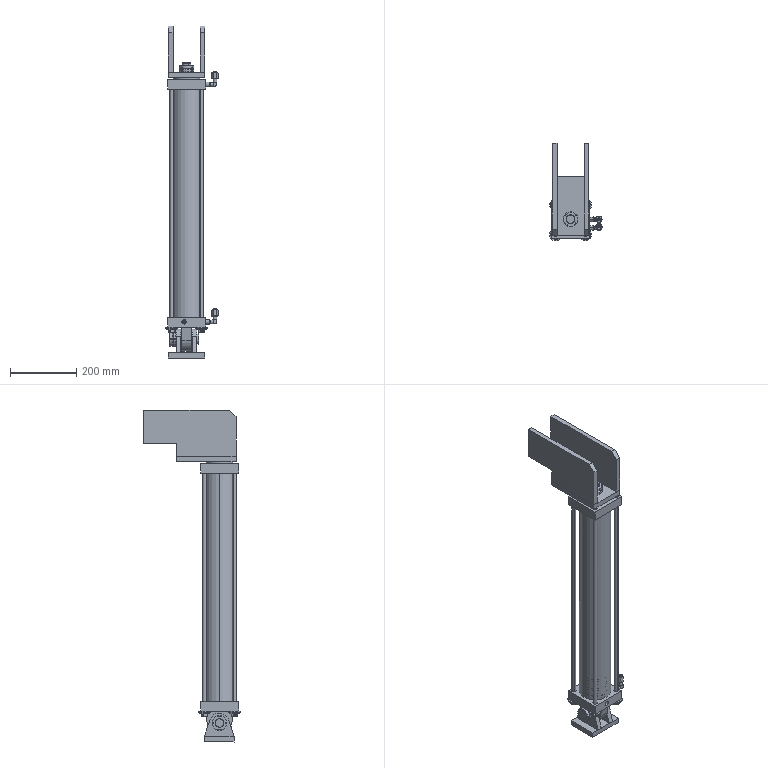Part | SolidWorks | features MirrorCompFeat 2, ReferencePattern 2 | 31 solids | 792 faces | box 159.892 x 293.5 x 1004 mm | volume 4407158 mm3 | cylinder 300 | plane 295 | cone 171 | torus 18 | sphere 6 | spline 2 | commonest cylinder face diameters 3.2 x32 6 x25 90 x18 12.5 x16 45 x16 4 x12